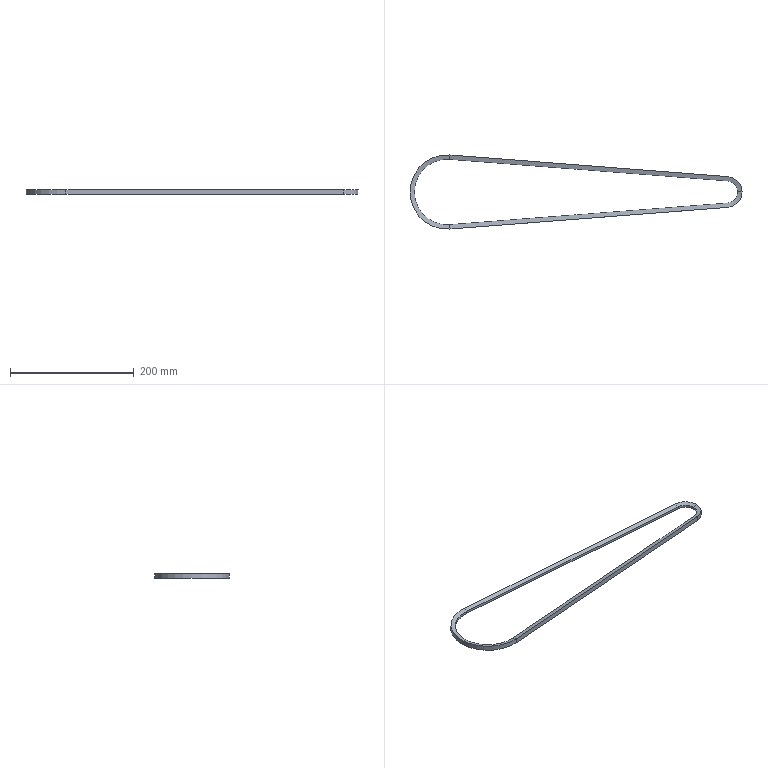Part | NX | features BREP 1 | 1 solid | 18 faces | box 536.48 x 119.96 x 8 mm | volume 48431 mm3 | plane 8 | cone 6 | cylinder 4 | commonest cylinder face diameters 35.96 x1 49.96 x1 105.96 x1 119.96 x1
STEP:
#1=CARTESIAN_POINT('',(4.107,52.821,-2.));
#2=VERTEX_POINT('',#1);
#3=CARTESIAN_POINT('',(-52.98,0.,-2.));
#4=VERTEX_POINT('',#3);
#5=CARTESIAN_POINT('',(0.,0.,-2.));
#6=DIRECTION('',(0.,0.,1.));
#7=DIRECTION('',(1.,0.,0.));
#8=AXIS2_PLACEMENT_3D('',#5,#6,#7);
#9=CIRCLE('',#8,52.98);
#10=EDGE_CURVE('',#2,#4,#9,.T.);
#11=ORIENTED_EDGE('',*,*,#10,.T.);
#12=CARTESIAN_POINT('',(-59.98,0.,-4.));
#13=VERTEX_POINT('',#12);
#14=CARTESIAN_POINT('',(-52.98,0.,-2.));
#15=DIRECTION('',(-0.9615,0.,-0.2747));
#16=VECTOR('',#15,1000.);
#17=LINE('',#14,#16);
#18=EDGE_CURVE('',#4,#13,#17,.T.);
#19=ORIENTED_EDGE('',*,*,#18,.T.);
#20=CARTESIAN_POINT('',(4.649,59.8,-4.));
#21=VERTEX_POINT('',#20);
#22=CARTESIAN_POINT('',(0.,0.,-4.));
#23=DIRECTION('',(0.,0.,1.));
#24=DIRECTION('',(1.,0.,0.));
#25=AXIS2_PLACEMENT_3D('',#22,#23,#24);
#26=CIRCLE('',#25,59.98);
#27=EDGE_CURVE('',#21,#13,#26,.T.);
#28=ORIENTED_EDGE('',*,*,#27,.F.);
#29=CARTESIAN_POINT('',(4.107,52.821,-2.));
#30=DIRECTION('',(0.07453,0.9586,-0.2747));
#31=VECTOR('',#30,1000.);
#32=LINE('',#29,#31);
#33=EDGE_CURVE('',#2,#21,#32,.T.);
#34=ORIENTED_EDGE('',*,*,#33,.F.);
#35=EDGE_LOOP('',(#11,#19,#28,#34));
#36=FACE_BOUND('',#35,.T.);
#37=CARTESIAN_POINT('',(0.,0.,-2.));
#38=DIRECTION('',(0.,0.,-1.));
#39=DIRECTION('',(1.,0.,0.));
#40=AXIS2_PLACEMENT_3D('',#37,#38,#39);
#41=CONICAL_SURFACE('',#40,52.98,1.292);
#42=ADVANCED_FACE('',(#36),#41,.F.);
#43=CARTESIAN_POINT('',(452.914,17.926,2.));
#44=VERTEX_POINT('',#43);
#45=CARTESIAN_POINT('',(469.5,0.,2.));
#46=VERTEX_POINT('',#45);
#47=CARTESIAN_POINT('',(451.52,0.,2.));
#48=DIRECTION('',(0.,0.,-1.));
#49=DIRECTION('',(-1.,0.,0.));
#50=AXIS2_PLACEMENT_3D('',#47,#48,#49);
#51=CIRCLE('',#50,17.98);
#52=EDGE_CURVE('',#44,#46,#51,.T.);
#53=ORIENTED_EDGE('',*,*,#52,.T.);
#54=CARTESIAN_POINT('',(476.5,0.,4.));
#55=VERTEX_POINT('',#54);
#56=CARTESIAN_POINT('',(476.5,0.,4.));
#57=DIRECTION('',(0.9615,0.,0.2747));
#58=VECTOR('',#57,1000.);
#59=LINE('',#56,#58);
#60=EDGE_CURVE('',#46,#55,#59,.T.);
#61=ORIENTED_EDGE('',*,*,#60,.T.);
#62=CARTESIAN_POINT('',(453.456,24.905,4.));
#63=VERTEX_POINT('',#62);
#64=CARTESIAN_POINT('',(451.52,0.,4.));
#65=DIRECTION('',(0.,0.,-1.));
#66=DIRECTION('',(-1.,0.,0.));
#67=AXIS2_PLACEMENT_3D('',#64,#65,#66);
#68=CIRCLE('',#67,24.98);
#69=EDGE_CURVE('',#63,#55,#68,.T.);
#70=ORIENTED_EDGE('',*,*,#69,.F.);
#71=CARTESIAN_POINT('',(452.914,17.926,2.));
#72=DIRECTION('',(-0.07453,-0.9586,-0.2747));
#73=VECTOR('',#72,1000.);
#74=LINE('',#71,#73);
#75=EDGE_CURVE('',#63,#44,#74,.T.);
#76=ORIENTED_EDGE('',*,*,#75,.T.);
#77=EDGE_LOOP('',(#53,#61,#70,#76));
#78=FACE_BOUND('',#77,.T.);
#79=CARTESIAN_POINT('',(451.52,0.,4.));
#80=DIRECTION('',(0.,0.,1.));
#81=DIRECTION('',(-1.,0.,0.));
#82=AXIS2_PLACEMENT_3D('',#79,#80,#81);
#83=CONICAL_SURFACE('',#82,24.98,1.292);
#84=ADVANCED_FACE('',(#78),#83,.F.);
#85=CARTESIAN_POINT('',(452.914,-17.926,2.));
#86=VERTEX_POINT('',#85);
#87=CARTESIAN_POINT('',(452.914,-17.926,-2.));
#88=VERTEX_POINT('',#87);
#89=CARTESIAN_POINT('',(452.914,-17.926,2.));
#90=DIRECTION('',(0.,0.,-1.));
#91=VECTOR('',#90,1000.);
#92=LINE('',#89,#91);
#93=EDGE_CURVE('',#86,#88,#92,.T.);
#94=ORIENTED_EDGE('',*,*,#93,.T.);
#95=CARTESIAN_POINT('',(4.107,-52.821,-2.));
#96=VERTEX_POINT('',#95);
#97=CARTESIAN_POINT('',(452.914,-17.926,-2.));
#98=DIRECTION('',(-0.997,-0.07752,0.));
#99=VECTOR('',#98,1000.);
#100=LINE('',#97,#99);
#101=EDGE_CURVE('',#88,#96,#100,.T.);
#102=ORIENTED_EDGE('',*,*,#101,.T.);
#103=CARTESIAN_POINT('',(4.107,-52.821,2.));
#104=VERTEX_POINT('',#103);
#105=CARTESIAN_POINT('',(4.107,-52.821,2.));
#106=DIRECTION('',(0.,0.,-1.));
#107=VECTOR('',#106,1000.);
#108=LINE('',#105,#107);
#109=EDGE_CURVE('',#104,#96,#108,.T.);
#110=ORIENTED_EDGE('',*,*,#109,.F.);
#111=CARTESIAN_POINT('',(452.914,-17.926,2.));
#112=DIRECTION('',(-0.997,-0.07752,0.));
#113=VECTOR('',#112,1000.);
#114=LINE('',#111,#113);
#115=EDGE_CURVE('',#86,#104,#114,.T.);
#116=ORIENTED_EDGE('',*,*,#115,.F.);
#117=EDGE_LOOP('',(#94,#102,#110,#116));
#118=FACE_BOUND('',#117,.T.);
#119=CARTESIAN_POINT('',(452.914,-17.926,2.));
#120=DIRECTION('',(-0.07752,0.997,0.));
#121=DIRECTION('',(0.,0.,-1.));
#122=AXIS2_PLACEMENT_3D('',#119,#120,#121);
#123=PLANE('',#122);
#124=ADVANCED_FACE('',(#118),#123,.T.);
#125=CARTESIAN_POINT('',(453.456,-24.905,-4.));
#126=VERTEX_POINT('',#125);
#127=CARTESIAN_POINT('',(452.914,-17.926,-2.));
#128=DIRECTION('',(0.07453,-0.9586,-0.2747));
#129=VECTOR('',#128,1000.);
#130=LINE('',#127,#129);
#131=EDGE_CURVE('',#88,#126,#130,.T.);
#132=ORIENTED_EDGE('',*,*,#131,.T.);
#133=CARTESIAN_POINT('',(4.649,-59.8,-4.));
#134=VERTEX_POINT('',#133);
#135=CARTESIAN_POINT('',(453.456,-24.905,-4.));
#136=DIRECTION('',(-0.997,-0.07752,0.));
#137=VECTOR('',#136,1000.);
#138=LINE('',#135,#137);
#139=EDGE_CURVE('',#126,#134,#138,.T.);
#140=ORIENTED_EDGE('',*,*,#139,.T.);
#141=CARTESIAN_POINT('',(4.107,-52.821,-2.));
#142=DIRECTION('',(0.07453,-0.9586,-0.2747));
#143=VECTOR('',#142,1000.);
#144=LINE('',#141,#143);
#145=EDGE_CURVE('',#96,#134,#144,.T.);
#146=ORIENTED_EDGE('',*,*,#145,.F.);
#147=ORIENTED_EDGE('',*,*,#101,.F.);
#148=EDGE_LOOP('',(#132,#140,#146,#147));
#149=FACE_BOUND('',#148,.T.);
#150=CARTESIAN_POINT('',(452.914,-17.926,-2.));
#151=DIRECTION('',(-0.0213,0.2739,-0.9615));
#152=DIRECTION('',(0.9998,0.,-0.02214));
#153=AXIS2_PLACEMENT_3D('',#150,#151,#152);
#154=PLANE('',#153);
#155=ADVANCED_FACE('',(#149),#154,.T.);
#156=CARTESIAN_POINT('',(453.456,-24.905,4.));
#157=VERTEX_POINT('',#156);
#158=CARTESIAN_POINT('',(453.456,-24.905,-4.));
#159=DIRECTION('',(0.,0.,1.));
#160=VECTOR('',#159,1000.);
#161=LINE('',#158,#160);
#162=EDGE_CURVE('',#126,#157,#161,.T.);
#163=ORIENTED_EDGE('',*,*,#162,.T.);
#164=CARTESIAN_POINT('',(4.649,-59.8,4.));
#165=VERTEX_POINT('',#164);
#166=CARTESIAN_POINT('',(453.456,-24.905,4.));
#167=DIRECTION('',(-0.997,-0.07752,0.));
#168=VECTOR('',#167,1000.);
#169=LINE('',#166,#168);
#170=EDGE_CURVE('',#157,#165,#169,.T.);
#171=ORIENTED_EDGE('',*,*,#170,.T.);
#172=CARTESIAN_POINT('',(4.649,-59.8,-4.));
#173=DIRECTION('',(0.,0.,1.));
#174=VECTOR('',#173,1000.);
#175=LINE('',#172,#174);
#176=EDGE_CURVE('',#134,#165,#175,.T.);
#177=ORIENTED_EDGE('',*,*,#176,.F.);
#178=ORIENTED_EDGE('',*,*,#139,.F.);
#179=EDGE_LOOP('',(#163,#171,#177,#178));
#180=FACE_BOUND('',#179,.T.);
#181=CARTESIAN_POINT('',(453.456,-24.905,-4.));
#182=DIRECTION('',(0.07752,-0.997,0.));
#183=DIRECTION('',(0.,0.,1.));
#184=AXIS2_PLACEMENT_3D('',#181,#182,#183);
#185=PLANE('',#184);
#186=ADVANCED_FACE('',(#180),#185,.T.);
#187=CARTESIAN_POINT('',(452.914,-17.926,2.));
#188=DIRECTION('',(-0.07453,0.9586,-0.2747));
#189=VECTOR('',#188,1000.);
#190=LINE('',#187,#189);
#191=EDGE_CURVE('',#157,#86,#190,.T.);
#192=ORIENTED_EDGE('',*,*,#191,.T.);
#193=ORIENTED_EDGE('',*,*,#115,.T.);
#194=CARTESIAN_POINT('',(4.107,-52.821,2.));
#195=DIRECTION('',(-0.07453,0.9586,-0.2747));
#196=VECTOR('',#195,1000.);
#197=LINE('',#194,#196);
#198=EDGE_CURVE('',#165,#104,#197,.T.);
#199=ORIENTED_EDGE('',*,*,#198,.F.);
#200=ORIENTED_EDGE('',*,*,#170,.F.);
#201=EDGE_LOOP('',(#192,#193,#199,#200));
#202=FACE_BOUND('',#201,.T.);
#203=CARTESIAN_POINT('',(452.914,-17.926,2.));
#204=DIRECTION('',(-0.0213,0.2739,0.9615));
#205=DIRECTION('',(-0.997,-0.07752,0.));
#206=AXIS2_PLACEMENT_3D('',#203,#204,#205);
#207=PLANE('',#206);
#208=ADVANCED_FACE('',(#202),#207,.T.);
#209=CARTESIAN_POINT('',(452.914,17.926,-2.));
#210=VERTEX_POINT('',#209);
#211=CARTESIAN_POINT('',(452.914,17.926,2.));
#212=DIRECTION('',(0.,0.,-1.));
#213=VECTOR('',#212,1000.);
#214=LINE('',#211,#213);
#215=EDGE_CURVE('',#44,#210,#214,.T.);
#216=ORIENTED_EDGE('',*,*,#215,.T.);
#217=CARTESIAN_POINT('',(451.52,0.,-2.));
#218=DIRECTION('',(0.,0.,-1.));
#219=DIRECTION('',(-1.,0.,0.));
#220=AXIS2_PLACEMENT_3D('',#217,#218,#219);
#221=CIRCLE('',#220,17.98);
#222=EDGE_CURVE('',#210,#88,#221,.T.);
#223=ORIENTED_EDGE('',*,*,#222,.T.);
#224=ORIENTED_EDGE('',*,*,#93,.F.);
#225=CARTESIAN_POINT('',(451.52,0.,2.));
#226=DIRECTION('',(0.,0.,-1.));
#227=DIRECTION('',(-1.,0.,0.));
#228=AXIS2_PLACEMENT_3D('',#225,#226,#227);
#229=CIRCLE('',#228,17.98);
#230=EDGE_CURVE('',#46,#86,#229,.T.);
#231=ORIENTED_EDGE('',*,*,#230,.F.);
#232=ORIENTED_EDGE('',*,*,#52,.F.);
#233=EDGE_LOOP('',(#216,#223,#224,#231,#232));
#234=FACE_BOUND('',#233,.T.);
#235=CARTESIAN_POINT('',(451.52,0.,0.));
#236=DIRECTION('',(0.,0.,-1.));
#237=DIRECTION('',(1.,0.,0.));
#238=AXIS2_PLACEMENT_3D('',#235,#236,#237);
#239=CYLINDRICAL_SURFACE('',#238,17.98);
#240=ADVANCED_FACE('',(#234),#239,.F.);
#241=CARTESIAN_POINT('',(453.456,24.905,-4.));
#242=VERTEX_POINT('',#241);
#243=CARTESIAN_POINT('',(452.914,17.926,-2.));
#244=DIRECTION('',(0.07453,0.9586,-0.2747));
#245=VECTOR('',#244,1000.);
#246=LINE('',#243,#245);
#247=EDGE_CURVE('',#210,#242,#246,.T.);
#248=ORIENTED_EDGE('',*,*,#247,.T.);
#249=CARTESIAN_POINT('',(451.52,0.,-4.));
#250=DIRECTION('',(0.,0.,-1.));
#251=DIRECTION('',(-1.,0.,0.));
#252=AXIS2_PLACEMENT_3D('',#249,#250,#251);
#253=CIRCLE('',#252,24.98);
#254=EDGE_CURVE('',#242,#126,#253,.T.);
#255=ORIENTED_EDGE('',*,*,#254,.T.);
#256=ORIENTED_EDGE('',*,*,#131,.F.);
#257=ORIENTED_EDGE('',*,*,#222,.F.);
#258=EDGE_LOOP('',(#248,#255,#256,#257));
#259=FACE_BOUND('',#258,.T.);
#260=CARTESIAN_POINT('',(451.52,0.,-2.));
#261=DIRECTION('',(0.,0.,-1.));
#262=DIRECTION('',(1.,0.,0.));
#263=AXIS2_PLACEMENT_3D('',#260,#261,#262);
#264=CONICAL_SURFACE('',#263,17.98,1.292);
#265=ADVANCED_FACE('',(#259),#264,.F.);
#266=CARTESIAN_POINT('',(453.456,24.905,-4.));
#267=DIRECTION('',(0.,0.,1.));
#268=VECTOR('',#267,1000.);
#269=LINE('',#266,#268);
#270=EDGE_CURVE('',#242,#63,#269,.T.);
#271=ORIENTED_EDGE('',*,*,#270,.T.);
#272=ORIENTED_EDGE('',*,*,#69,.T.);
#273=CARTESIAN_POINT('',(451.52,0.,4.));
#274=DIRECTION('',(0.,0.,-1.));
#275=DIRECTION('',(-1.,0.,0.));
#276=AXIS2_PLACEMENT_3D('',#273,#274,#275);
#277=CIRCLE('',#276,24.98);
#278=EDGE_CURVE('',#55,#157,#277,.T.);
#279=ORIENTED_EDGE('',*,*,#278,.T.);
#280=ORIENTED_EDGE('',*,*,#162,.F.);
#281=ORIENTED_EDGE('',*,*,#254,.F.);
#282=EDGE_LOOP('',(#271,#272,#279,#280,#281));
#283=FACE_BOUND('',#282,.T.);
#284=CARTESIAN_POINT('',(451.52,0.,0.));
#285=DIRECTION('',(0.,0.,-1.));
#286=DIRECTION('',(1.,0.,0.));
#287=AXIS2_PLACEMENT_3D('',#284,#285,#286);
#288=CYLINDRICAL_SURFACE('',#287,24.98);
#289=ADVANCED_FACE('',(#283),#288,.T.);
#290=ORIENTED_EDGE('',*,*,#60,.F.);
#291=ORIENTED_EDGE('',*,*,#230,.T.);
#292=ORIENTED_EDGE('',*,*,#191,.F.);
#293=ORIENTED_EDGE('',*,*,#278,.F.);
#294=EDGE_LOOP('',(#290,#291,#292,#293));
#295=FACE_BOUND('',#294,.T.);
#296=CARTESIAN_POINT('',(451.52,0.,4.));
#297=DIRECTION('',(0.,0.,1.));
#298=DIRECTION('',(-1.,0.,0.));
#299=AXIS2_PLACEMENT_3D('',#296,#297,#298);
#300=CONICAL_SURFACE('',#299,24.98,1.292);
#301=ADVANCED_FACE('',(#295),#300,.F.);
#302=CARTESIAN_POINT('',(4.107,52.821,2.));
#303=VERTEX_POINT('',#302);
#304=CARTESIAN_POINT('',(4.107,52.821,2.));
#305=DIRECTION('',(0.,0.,-1.));
#306=VECTOR('',#305,1000.);
#307=LINE('',#304,#306);
#308=EDGE_CURVE('',#303,#2,#307,.T.);
#309=ORIENTED_EDGE('',*,*,#308,.T.);
#310=CARTESIAN_POINT('',(4.107,52.821,-2.));
#311=DIRECTION('',(0.997,-0.07752,0.));
#312=VECTOR('',#311,1000.);
#313=LINE('',#310,#312);
#314=EDGE_CURVE('',#2,#210,#313,.T.);
#315=ORIENTED_EDGE('',*,*,#314,.T.);
#316=ORIENTED_EDGE('',*,*,#215,.F.);
#317=CARTESIAN_POINT('',(4.107,52.821,2.));
#318=DIRECTION('',(0.997,-0.07752,0.));
#319=VECTOR('',#318,1000.);
#320=LINE('',#317,#319);
#321=EDGE_CURVE('',#303,#44,#320,.T.);
#322=ORIENTED_EDGE('',*,*,#321,.F.);
#323=EDGE_LOOP('',(#309,#315,#316,#322));
#324=FACE_BOUND('',#323,.T.);
#325=CARTESIAN_POINT('',(4.107,52.821,2.));
#326=DIRECTION('',(-0.07752,-0.997,0.));
#327=DIRECTION('',(0.997,-0.07752,0.));
#328=AXIS2_PLACEMENT_3D('',#325,#326,#327);
#329=PLANE('',#328);
#330=ADVANCED_FACE('',(#324),#329,.T.);
#331=ORIENTED_EDGE('',*,*,#33,.T.);
#332=CARTESIAN_POINT('',(4.649,59.8,-4.));
#333=DIRECTION('',(0.997,-0.07752,0.));
#334=VECTOR('',#333,1000.);
#335=LINE('',#332,#334);
#336=EDGE_CURVE('',#21,#242,#335,.T.);
#337=ORIENTED_EDGE('',*,*,#336,.T.);
#338=ORIENTED_EDGE('',*,*,#247,.F.);
#339=ORIENTED_EDGE('',*,*,#314,.F.);
#340=EDGE_LOOP('',(#331,#337,#338,#339));
#341=FACE_BOUND('',#340,.T.);
#342=CARTESIAN_POINT('',(4.107,52.821,-2.));
#343=DIRECTION('',(-0.0213,-0.2739,-0.9615));
#344=DIRECTION('',(0.,0.9617,-0.274));
#345=AXIS2_PLACEMENT_3D('',#342,#343,#344);
#346=PLANE('',#345);
#347=ADVANCED_FACE('',(#341),#346,.T.);
#348=CARTESIAN_POINT('',(4.649,59.8,4.));
#349=VERTEX_POINT('',#348);
#350=CARTESIAN_POINT('',(4.649,59.8,-4.));
#351=DIRECTION('',(0.,0.,1.));
#352=VECTOR('',#351,1000.);
#353=LINE('',#350,#352);
#354=EDGE_CURVE('',#21,#349,#353,.T.);
#355=ORIENTED_EDGE('',*,*,#354,.T.);
#356=CARTESIAN_POINT('',(4.649,59.8,4.));
#357=DIRECTION('',(0.997,-0.07752,0.));
#358=VECTOR('',#357,1000.);
#359=LINE('',#356,#358);
#360=EDGE_CURVE('',#349,#63,#359,.T.);
#361=ORIENTED_EDGE('',*,*,#360,.T.);
#362=ORIENTED_EDGE('',*,*,#270,.F.);
#363=ORIENTED_EDGE('',*,*,#336,.F.);
#364=EDGE_LOOP('',(#355,#361,#362,#363));
#365=FACE_BOUND('',#364,.T.);
#366=CARTESIAN_POINT('',(4.649,59.8,-4.));
#367=DIRECTION('',(0.07752,0.997,0.));
#368=DIRECTION('',(0.,0.,1.));
#369=AXIS2_PLACEMENT_3D('',#366,#367,#368);
#370=PLANE('',#369);
#371=ADVANCED_FACE('',(#365),#370,.T.);
#372=CARTESIAN_POINT('',(4.107,52.821,2.));
#373=DIRECTION('',(-0.07453,-0.9586,-0.2747));
#374=VECTOR('',#373,1000.);
#375=LINE('',#372,#374);
#376=EDGE_CURVE('',#349,#303,#375,.T.);
#377=ORIENTED_EDGE('',*,*,#376,.T.);
#378=ORIENTED_EDGE('',*,*,#321,.T.);
#379=ORIENTED_EDGE('',*,*,#75,.F.);
#380=ORIENTED_EDGE('',*,*,#360,.F.);
#381=EDGE_LOOP('',(#377,#378,#379,#380));
#382=FACE_BOUND('',#381,.T.);
#383=CARTESIAN_POINT('',(4.107,52.821,2.));
#384=DIRECTION('',(-0.0213,-0.2739,0.9615));
#385=DIRECTION('',(0.997,-0.07752,0.));
#386=AXIS2_PLACEMENT_3D('',#383,#384,#385);
#387=PLANE('',#386);
#388=ADVANCED_FACE('',(#382),#387,.T.);
#389=CARTESIAN_POINT('',(0.,0.,2.));
#390=DIRECTION('',(0.,0.,1.));
#391=DIRECTION('',(1.,0.,0.));
#392=AXIS2_PLACEMENT_3D('',#389,#390,#391);
#393=CIRCLE('',#392,52.98);
#394=EDGE_CURVE('',#303,#104,#393,.T.);
#395=ORIENTED_EDGE('',*,*,#394,.F.);
#396=ORIENTED_EDGE('',*,*,#376,.F.);
#397=CARTESIAN_POINT('',(0.,0.,4.));
#398=DIRECTION('',(0.,0.,1.));
#399=DIRECTION('',(1.,0.,0.));
#400=AXIS2_PLACEMENT_3D('',#397,#398,#399);
#401=CIRCLE('',#400,59.98);
#402=EDGE_CURVE('',#349,#165,#401,.T.);
#403=ORIENTED_EDGE('',*,*,#402,.T.);
#404=ORIENTED_EDGE('',*,*,#198,.T.);
#405=EDGE_LOOP('',(#395,#396,#403,#404));
#406=FACE_BOUND('',#405,.T.);
#407=CARTESIAN_POINT('',(0.,0.,4.));
#408=DIRECTION('',(0.,0.,1.));
#409=DIRECTION('',(-1.,0.,0.));
#410=AXIS2_PLACEMENT_3D('',#407,#408,#409);
#411=CONICAL_SURFACE('',#410,59.98,1.292);
#412=ADVANCED_FACE('',(#406),#411,.F.);
#413=ORIENTED_EDGE('',*,*,#10,.F.);
#414=ORIENTED_EDGE('',*,*,#308,.F.);
#415=ORIENTED_EDGE('',*,*,#394,.T.);
#416=ORIENTED_EDGE('',*,*,#109,.T.);
#417=CARTESIAN_POINT('',(0.,0.,-2.));
#418=DIRECTION('',(0.,0.,1.));
#419=DIRECTION('',(1.,0.,0.));
#420=AXIS2_PLACEMENT_3D('',#417,#418,#419);
#421=CIRCLE('',#420,52.98);
#422=EDGE_CURVE('',#4,#96,#421,.T.);
#423=ORIENTED_EDGE('',*,*,#422,.F.);
#424=EDGE_LOOP('',(#413,#414,#415,#416,#423));
#425=FACE_BOUND('',#424,.T.);
#426=CARTESIAN_POINT('',(0.,0.,0.));
#427=DIRECTION('',(0.,0.,1.));
#428=DIRECTION('',(-1.,0.,0.));
#429=AXIS2_PLACEMENT_3D('',#426,#427,#428);
#430=CYLINDRICAL_SURFACE('',#429,52.98);
#431=ADVANCED_FACE('',(#425),#430,.F.);
#432=ORIENTED_EDGE('',*,*,#18,.F.);
#433=ORIENTED_EDGE('',*,*,#422,.T.);
#434=ORIENTED_EDGE('',*,*,#145,.T.);
#435=CARTESIAN_POINT('',(0.,0.,-4.));
#436=DIRECTION('',(0.,0.,1.));
#437=DIRECTION('',(1.,0.,0.));
#438=AXIS2_PLACEMENT_3D('',#435,#436,#437);
#439=CIRCLE('',#438,59.98);
#440=EDGE_CURVE('',#13,#134,#439,.T.);
#441=ORIENTED_EDGE('',*,*,#440,.F.);
#442=EDGE_LOOP('',(#432,#433,#434,#441));
#443=FACE_BOUND('',#442,.T.);
#444=CARTESIAN_POINT('',(0.,0.,-2.));
#445=DIRECTION('',(0.,0.,-1.));
#446=DIRECTION('',(1.,0.,0.));
#447=AXIS2_PLACEMENT_3D('',#444,#445,#446);
#448=CONICAL_SURFACE('',#447,52.98,1.292);
#449=ADVANCED_FACE('',(#443),#448,.F.);
#450=ORIENTED_EDGE('',*,*,#354,.F.);
#451=ORIENTED_EDGE('',*,*,#27,.T.);
#452=ORIENTED_EDGE('',*,*,#440,.T.);
#453=ORIENTED_EDGE('',*,*,#176,.T.);
#454=ORIENTED_EDGE('',*,*,#402,.F.);
#455=EDGE_LOOP('',(#450,#451,#452,#453,#454));
#456=FACE_BOUND('',#455,.T.);
#457=CARTESIAN_POINT('',(0.,0.,0.));
#458=DIRECTION('',(0.,0.,1.));
#459=DIRECTION('',(-1.,0.,0.));
#460=AXIS2_PLACEMENT_3D('',#457,#458,#459);
#461=CYLINDRICAL_SURFACE('',#460,59.98);
#462=ADVANCED_FACE('',(#456),#461,.T.);
#463=CLOSED_SHELL('',(#42,#84,#124,#155,#186,#208,#240,#265,#289,#301,#330,#347,#371,#388,#412,#431,#449,#462));
#464=MANIFOLD_SOLID_BREP('',#463);
#465=(LENGTH_UNIT()NAMED_UNIT(*)SI_UNIT(.MILLI.,.METRE.));
#466=UNCERTAINTY_MEASURE_WITH_UNIT(LENGTH_MEASURE(0.00001),#465,'','');
#467=(NAMED_UNIT(*)PLANE_ANGLE_UNIT()SI_UNIT($,.RADIAN.));
#468=(NAMED_UNIT(*)SI_UNIT($,.STERADIAN.)SOLID_ANGLE_UNIT());
#469=(GEOMETRIC_REPRESENTATION_CONTEXT(3)GLOBAL_UNCERTAINTY_ASSIGNED_CONTEXT((#466))GLOBAL_UNIT_ASSIGNED_CONTEXT((#465,#467,#468))REPRESENTATION_CONTEXT('',''));
#470=ADVANCED_BREP_SHAPE_REPRESENTATION('',(#464),#469);